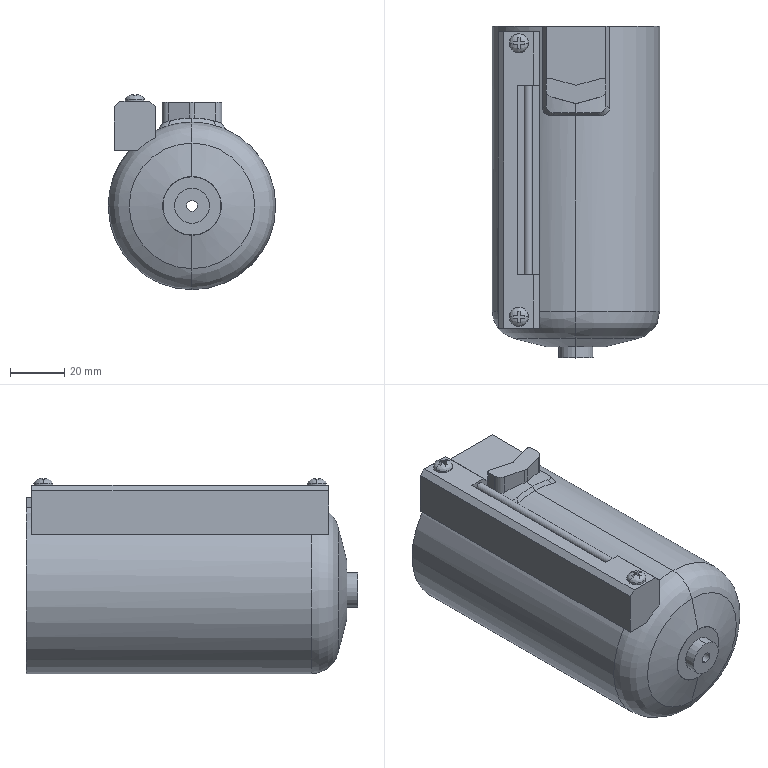Part | STEP file | AC40-04-KSTV-38JNR_AC3009A AF Bowl-2 | 1 solid | 93 faces | box 61.5 x 121.9 x 71.711 mm | volume 50188 mm3 | plane 53 | cylinder 22 | spline 6 | cone 6 | torus 6 | commonest cylinder face diameters 7 x4 2 x3 6 x3 3 x2 4 x2 12.8 x2